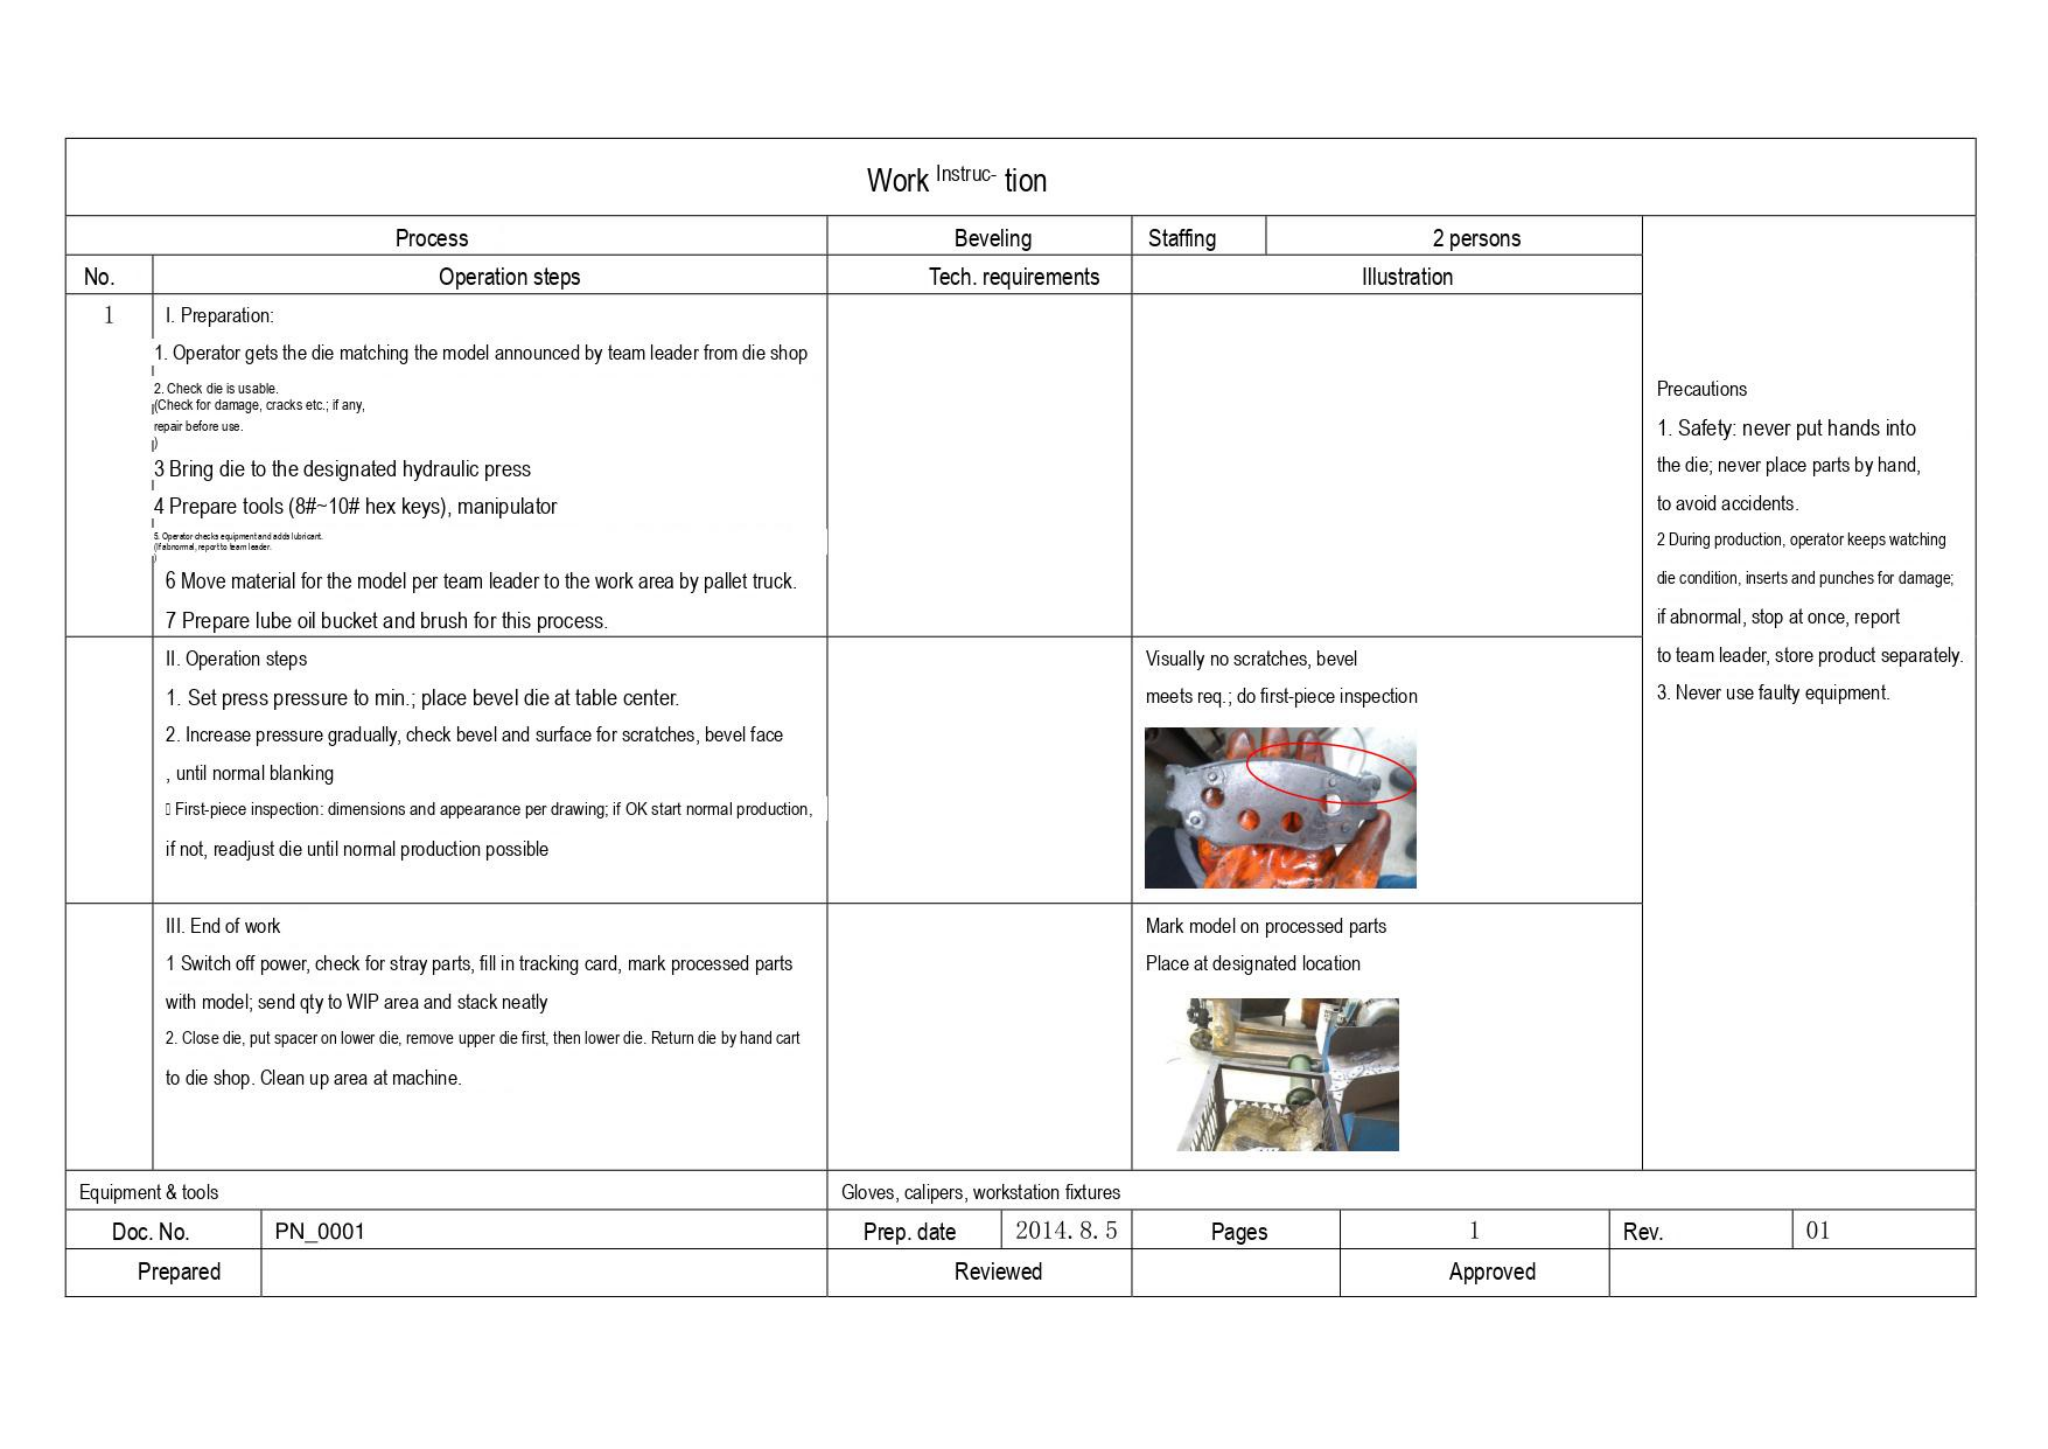# Work Instruc- tion

| Process | | Beveling | Staffing | 2 persons |
|---|---|---|---|---|

| No. | Operation steps | Tech. requirements | Illustration | Precautions |
|---|---|---|---|---|
| 1 | I. Preparation:<br>1. Operator gets the die matching the model announced by team leader from die shop<br>2. Check die is usable.<br>(Check for damage, cracks etc.; if any, repair before use.<br>)<br>3 Bring die to the designated hydraulic press<br>4 Prepare tools (8#~10# hex keys), manipulator<br>5. Operator checks equipment and adds lubricant.<br>(If abnormal, report to team leader.<br>)<br>6 Move material for the model per team leader to the work area by pallet truck.<br>7 Prepare lube oil bucket and brush for this process. | | | Precautions<br>1. Safety: never put hands into the die; never place parts by hand, to avoid accidents.<br>2 During production, operator keeps watching die condition, inserts and punches for damage; if abnormal, stop at once, report to team leader, store product separately.<br>3. Never use faulty equipment. |
| | II. Operation steps<br>1. Set press pressure to min.; place bevel die at table center.<br>2. Increase pressure gradually, check bevel and surface for scratches, bevel face , until normal blanking<br>▯ First-piece inspection: dimensions and appearance per drawing; if OK start normal production, if not, readjust die until normal production possible | | Visually no scratches, bevel meets req.; do first-piece inspection | |
| | III. End of work<br>1 Switch off power, check for stray parts, fill in tracking card, mark processed parts with model; send qty to WIP area and stack neatly<br>2. Close die, put spacer on lower die, remove upper die first, then lower die. Return die by hand cart to die shop. Clean up area at machine. | | Mark model on processed parts<br>Place at designated location | |

| Equipment & tools | Gloves, calipers, workstation fixtures |
|---|---|

| Doc. No. | PN_0001 | Prep. date | 2014. 8. 5 | Pages | 1 | Rev. | 01 |
|---|---|---|---|---|---|---|---|
| Prepared | | Reviewed | | Approved | | | |